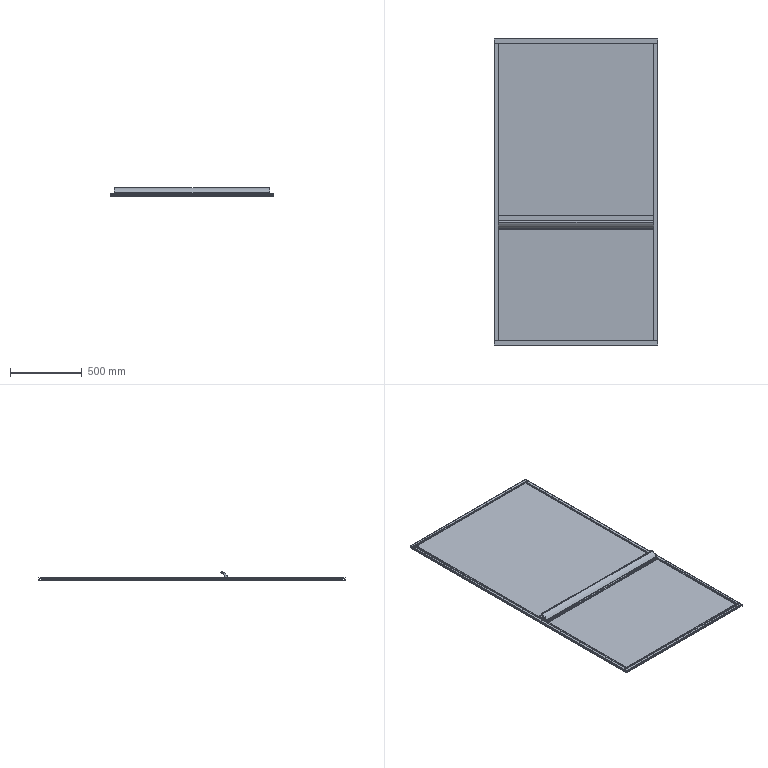Part | SolidWorks | features ICE 7, MirrorSolid 1, WeldMemberFeat 1, WeldmentFeature 1 | 13 solids | 408 faces | box 1140 x 2136 x 62.186 mm | volume 24296668 mm3 | plane 252 | cylinder 156 | commonest cylinder face diameters 1.1 x36 3.6 x32 5.8 x29 4 x24 1 x10 0.4 x8